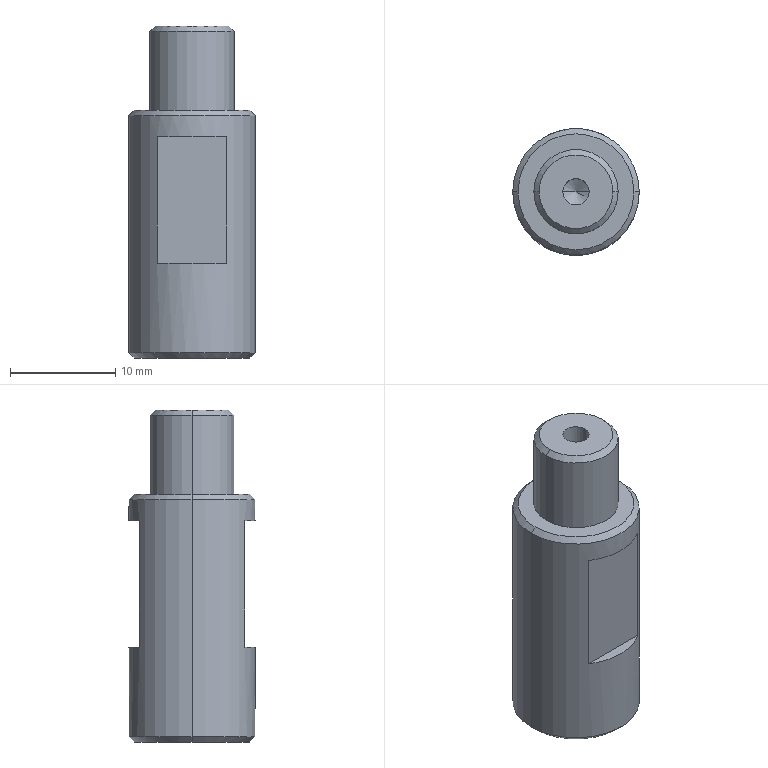Part | STEP file | 10000020542swp000-1 | 1 solid | 27 faces | box 12 x 12 x 31.5 mm | volume 2667 mm3 | cone 10 | plane 9 | cylinder 8 | commonest cylinder face diameters 2.5 x2 4.2 x2 8 x2 12 x2
STEP:
#1=CARTESIAN_POINT('',(3.5,0.,31.5));
#2=VERTEX_POINT('',#1);
#3=CARTESIAN_POINT('',(-3.5,0.,31.5));
#4=VERTEX_POINT('',#3);
#5=CARTESIAN_POINT('',(0.,0.,31.5));
#6=DIRECTION('',(0.,0.,1.));
#7=DIRECTION('',(1.,0.,0.));
#8=AXIS2_PLACEMENT_3D('',#5,#6,#7);
#9=CIRCLE('',#8,3.5);
#10=EDGE_CURVE('',#2,#4,#9,.T.);
#11=ORIENTED_EDGE('',*,*,#10,.F.);
#12=CARTESIAN_POINT('',(4.,0.,31.));
#13=VERTEX_POINT('',#12);
#14=CARTESIAN_POINT('',(3.5,0.,31.5));
#15=DIRECTION('',(0.7071,0.,-0.7071));
#16=VECTOR('',#15,1000.);
#17=LINE('',#14,#16);
#18=EDGE_CURVE('',#2,#13,#17,.T.);
#19=ORIENTED_EDGE('',*,*,#18,.T.);
#20=CARTESIAN_POINT('',(-4.,0.,31.));
#21=VERTEX_POINT('',#20);
#22=CARTESIAN_POINT('',(0.,0.,31.));
#23=DIRECTION('',(0.,0.,-1.));
#24=DIRECTION('',(1.,0.,0.));
#25=AXIS2_PLACEMENT_3D('',#22,#23,#24);
#26=CIRCLE('',#25,4.);
#27=EDGE_CURVE('',#21,#13,#26,.T.);
#28=ORIENTED_EDGE('',*,*,#27,.F.);
#29=CARTESIAN_POINT('',(-3.5,0.,31.5));
#30=DIRECTION('',(-0.7071,0.,-0.7071));
#31=VECTOR('',#30,1000.);
#32=LINE('',#29,#31);
#33=EDGE_CURVE('',#4,#21,#32,.T.);
#34=ORIENTED_EDGE('',*,*,#33,.F.);
#35=EDGE_LOOP('',(#11,#19,#28,#34));
#36=FACE_OUTER_BOUND('',#35,.T.);
#37=CARTESIAN_POINT('',(0.,0.,31.5));
#38=DIRECTION('',(0.,0.,-1.));
#39=DIRECTION('',(-1.,0.,0.));
#40=AXIS2_PLACEMENT_3D('',#37,#38,#39);
#41=CONICAL_SURFACE('',#40,3.5,0.7854);
#42=ADVANCED_FACE('',(#36),#41,.T.);
#43=CARTESIAN_POINT('',(5.5,0.,23.5));
#44=VERTEX_POINT('',#43);
#45=CARTESIAN_POINT('',(-5.5,0.,23.5));
#46=VERTEX_POINT('',#45);
#47=CARTESIAN_POINT('',(0.,0.,23.5));
#48=DIRECTION('',(0.,0.,1.));
#49=DIRECTION('',(1.,0.,0.));
#50=AXIS2_PLACEMENT_3D('',#47,#48,#49);
#51=CIRCLE('',#50,5.5);
#52=EDGE_CURVE('',#44,#46,#51,.T.);
#53=ORIENTED_EDGE('',*,*,#52,.F.);
#54=CARTESIAN_POINT('',(6.,0.,23.));
#55=VERTEX_POINT('',#54);
#56=CARTESIAN_POINT('',(5.5,0.,23.5));
#57=DIRECTION('',(0.7071,0.,-0.7071));
#58=VECTOR('',#57,1000.);
#59=LINE('',#56,#58);
#60=EDGE_CURVE('',#44,#55,#59,.T.);
#61=ORIENTED_EDGE('',*,*,#60,.T.);
#62=CARTESIAN_POINT('',(-6.,0.,23.));
#63=VERTEX_POINT('',#62);
#64=CARTESIAN_POINT('',(0.,0.,23.));
#65=DIRECTION('',(0.,0.,-1.));
#66=DIRECTION('',(1.,0.,0.));
#67=AXIS2_PLACEMENT_3D('',#64,#65,#66);
#68=CIRCLE('',#67,6.);
#69=EDGE_CURVE('',#63,#55,#68,.T.);
#70=ORIENTED_EDGE('',*,*,#69,.F.);
#71=CARTESIAN_POINT('',(-5.5,0.,23.5));
#72=DIRECTION('',(-0.7071,0.,-0.7071));
#73=VECTOR('',#72,1000.);
#74=LINE('',#71,#73);
#75=EDGE_CURVE('',#46,#63,#74,.T.);
#76=ORIENTED_EDGE('',*,*,#75,.F.);
#77=EDGE_LOOP('',(#53,#61,#70,#76));
#78=FACE_OUTER_BOUND('',#77,.T.);
#79=CARTESIAN_POINT('',(0.,0.,23.5));
#80=DIRECTION('',(0.,0.,-1.));
#81=DIRECTION('',(-1.,0.,0.));
#82=AXIS2_PLACEMENT_3D('',#79,#80,#81);
#83=CONICAL_SURFACE('',#82,5.5,0.7854);
#84=ADVANCED_FACE('',(#78),#83,.T.);
#85=CARTESIAN_POINT('',(-5.5,0.,0.));
#86=VERTEX_POINT('',#85);
#87=CARTESIAN_POINT('',(5.5,0.,0.));
#88=VERTEX_POINT('',#87);
#89=CARTESIAN_POINT('',(0.,0.,0.));
#90=DIRECTION('',(0.,0.,-1.));
#91=DIRECTION('',(1.,0.,0.));
#92=AXIS2_PLACEMENT_3D('',#89,#90,#91);
#93=CIRCLE('',#92,5.5);
#94=EDGE_CURVE('',#86,#88,#93,.T.);
#95=ORIENTED_EDGE('',*,*,#94,.F.);
#96=CARTESIAN_POINT('',(-6.,0.,0.5));
#97=VERTEX_POINT('',#96);
#98=CARTESIAN_POINT('',(-6.,0.,0.5));
#99=DIRECTION('',(-0.7071,0.,0.7071));
#100=VECTOR('',#99,1000.);
#101=LINE('',#98,#100);
#102=EDGE_CURVE('',#86,#97,#101,.T.);
#103=ORIENTED_EDGE('',*,*,#102,.T.);
#104=CARTESIAN_POINT('',(6.,0.,0.5));
#105=VERTEX_POINT('',#104);
#106=CARTESIAN_POINT('',(0.,0.,0.5));
#107=DIRECTION('',(0.,0.,1.));
#108=DIRECTION('',(1.,0.,0.));
#109=AXIS2_PLACEMENT_3D('',#106,#107,#108);
#110=CIRCLE('',#109,6.);
#111=EDGE_CURVE('',#105,#97,#110,.T.);
#112=ORIENTED_EDGE('',*,*,#111,.F.);
#113=CARTESIAN_POINT('',(6.,0.,0.5));
#114=DIRECTION('',(0.7071,0.,0.7071));
#115=VECTOR('',#114,1000.);
#116=LINE('',#113,#115);
#117=EDGE_CURVE('',#88,#105,#116,.T.);
#118=ORIENTED_EDGE('',*,*,#117,.F.);
#119=EDGE_LOOP('',(#95,#103,#112,#118));
#120=FACE_OUTER_BOUND('',#119,.T.);
#121=CARTESIAN_POINT('',(0.,0.,0.5));
#122=DIRECTION('',(0.,0.,1.));
#123=DIRECTION('',(1.,0.,0.));
#124=AXIS2_PLACEMENT_3D('',#121,#122,#123);
#125=CONICAL_SURFACE('',#124,6.,0.7854);
#126=ADVANCED_FACE('',(#120),#125,.T.);
#127=CARTESIAN_POINT('',(2.1,0.,14.4));
#128=VERTEX_POINT('',#127);
#129=CARTESIAN_POINT('',(-2.1,0.,14.4));
#130=VERTEX_POINT('',#129);
#131=CARTESIAN_POINT('',(0.,0.,14.4));
#132=DIRECTION('',(0.,0.,-1.));
#133=DIRECTION('',(-1.,0.,0.));
#134=AXIS2_PLACEMENT_3D('',#131,#132,#133);
#135=CIRCLE('',#134,2.1);
#136=EDGE_CURVE('',#128,#130,#135,.T.);
#137=ORIENTED_EDGE('',*,*,#136,.F.);
#138=CARTESIAN_POINT('',(2.1,0.,0.));
#139=VERTEX_POINT('',#138);
#140=CARTESIAN_POINT('',(2.1,0.,0.));
#141=DIRECTION('',(0.,0.,-1.));
#142=VECTOR('',#141,1000.);
#143=LINE('',#140,#142);
#144=EDGE_CURVE('',#128,#139,#143,.T.);
#145=ORIENTED_EDGE('',*,*,#144,.T.);
#146=CARTESIAN_POINT('',(-2.1,0.,0.));
#147=VERTEX_POINT('',#146);
#148=CARTESIAN_POINT('',(0.,0.,0.));
#149=DIRECTION('',(0.,0.,-1.));
#150=DIRECTION('',(-1.,0.,0.));
#151=AXIS2_PLACEMENT_3D('',#148,#149,#150);
#152=CIRCLE('',#151,2.1);
#153=EDGE_CURVE('',#139,#147,#152,.T.);
#154=ORIENTED_EDGE('',*,*,#153,.T.);
#155=CARTESIAN_POINT('',(-2.1,0.,0.));
#156=DIRECTION('',(0.,0.,-1.));
#157=VECTOR('',#156,1000.);
#158=LINE('',#155,#157);
#159=EDGE_CURVE('',#130,#147,#158,.T.);
#160=ORIENTED_EDGE('',*,*,#159,.F.);
#161=EDGE_LOOP('',(#137,#145,#154,#160));
#162=FACE_OUTER_BOUND('',#161,.T.);
#163=CARTESIAN_POINT('',(0.,0.,0.));
#164=DIRECTION('',(0.,0.,-1.));
#165=DIRECTION('',(-1.,0.,0.));
#166=AXIS2_PLACEMENT_3D('',#163,#164,#165);
#167=CYLINDRICAL_SURFACE('',#166,2.1);
#168=ADVANCED_FACE('',(#162),#167,.F.);
#169=CARTESIAN_POINT('',(0.,0.,15.662));
#170=VERTEX_POINT('',#169);
#171=CARTESIAN_POINT('',(-2.1,0.,14.4));
#172=DIRECTION('',(-0.8572,0.,-0.515));
#173=VECTOR('',#172,1000.);
#174=LINE('',#171,#173);
#175=EDGE_CURVE('',#170,#130,#174,.T.);
#176=ORIENTED_EDGE('',*,*,#175,.F.);
#177=CARTESIAN_POINT('',(2.1,0.,14.4));
#178=DIRECTION('',(0.8572,0.,-0.515));
#179=VECTOR('',#178,1000.);
#180=LINE('',#177,#179);
#181=EDGE_CURVE('',#170,#128,#180,.T.);
#182=ORIENTED_EDGE('',*,*,#181,.T.);
#183=ORIENTED_EDGE('',*,*,#136,.T.);
#184=EDGE_LOOP('',(#176,#182,#183));
#185=FACE_OUTER_BOUND('',#184,.T.);
#186=CARTESIAN_POINT('',(0.,0.,14.4));
#187=DIRECTION('',(0.,0.,-1.));
#188=DIRECTION('',(-1.,0.,0.));
#189=AXIS2_PLACEMENT_3D('',#186,#187,#188);
#190=CONICAL_SURFACE('',#189,2.1,1.03);
#191=ADVANCED_FACE('',(#185),#190,.F.);
#192=CARTESIAN_POINT('',(-1.25,0.,18.));
#193=VERTEX_POINT('',#192);
#194=CARTESIAN_POINT('',(1.25,0.,18.));
#195=VERTEX_POINT('',#194);
#196=CARTESIAN_POINT('',(0.,0.,18.));
#197=DIRECTION('',(0.,0.,1.));
#198=DIRECTION('',(1.,0.,0.));
#199=AXIS2_PLACEMENT_3D('',#196,#197,#198);
#200=CIRCLE('',#199,1.25);
#201=EDGE_CURVE('',#193,#195,#200,.T.);
#202=ORIENTED_EDGE('',*,*,#201,.F.);
#203=CARTESIAN_POINT('',(-1.25,0.,31.5));
#204=VERTEX_POINT('',#203);
#205=CARTESIAN_POINT('',(-1.25,0.,31.5));
#206=DIRECTION('',(0.,0.,1.));
#207=VECTOR('',#206,1000.);
#208=LINE('',#205,#207);
#209=EDGE_CURVE('',#193,#204,#208,.T.);
#210=ORIENTED_EDGE('',*,*,#209,.T.);
#211=CARTESIAN_POINT('',(1.25,0.,31.5));
#212=VERTEX_POINT('',#211);
#213=CARTESIAN_POINT('',(0.,0.,31.5));
#214=DIRECTION('',(0.,0.,1.));
#215=DIRECTION('',(1.,0.,0.));
#216=AXIS2_PLACEMENT_3D('',#213,#214,#215);
#217=CIRCLE('',#216,1.25);
#218=EDGE_CURVE('',#204,#212,#217,.T.);
#219=ORIENTED_EDGE('',*,*,#218,.T.);
#220=CARTESIAN_POINT('',(1.25,0.,31.5));
#221=DIRECTION('',(0.,0.,1.));
#222=VECTOR('',#221,1000.);
#223=LINE('',#220,#222);
#224=EDGE_CURVE('',#195,#212,#223,.T.);
#225=ORIENTED_EDGE('',*,*,#224,.F.);
#226=EDGE_LOOP('',(#202,#210,#219,#225));
#227=FACE_OUTER_BOUND('',#226,.T.);
#228=CARTESIAN_POINT('',(0.,0.,31.5));
#229=DIRECTION('',(0.,0.,1.));
#230=DIRECTION('',(1.,0.,0.));
#231=AXIS2_PLACEMENT_3D('',#228,#229,#230);
#232=CYLINDRICAL_SURFACE('',#231,1.25);
#233=ADVANCED_FACE('',(#227),#232,.F.);
#234=CARTESIAN_POINT('',(0.,0.,17.249));
#235=VERTEX_POINT('',#234);
#236=CARTESIAN_POINT('',(1.25,0.,18.));
#237=DIRECTION('',(0.8572,0.,0.515));
#238=VECTOR('',#237,1000.);
#239=LINE('',#236,#238);
#240=EDGE_CURVE('',#235,#195,#239,.T.);
#241=ORIENTED_EDGE('',*,*,#240,.F.);
#242=CARTESIAN_POINT('',(-1.25,0.,18.));
#243=DIRECTION('',(-0.8572,0.,0.515));
#244=VECTOR('',#243,1000.);
#245=LINE('',#242,#244);
#246=EDGE_CURVE('',#235,#193,#245,.T.);
#247=ORIENTED_EDGE('',*,*,#246,.T.);
#248=ORIENTED_EDGE('',*,*,#201,.T.);
#249=EDGE_LOOP('',(#241,#247,#248));
#250=FACE_OUTER_BOUND('',#249,.T.);
#251=CARTESIAN_POINT('',(0.,0.,18.));
#252=DIRECTION('',(0.,0.,1.));
#253=DIRECTION('',(1.,0.,0.));
#254=AXIS2_PLACEMENT_3D('',#251,#252,#253);
#255=CONICAL_SURFACE('',#254,1.25,1.03);
#256=ADVANCED_FACE('',(#250),#255,.F.);
#257=ORIENTED_EDGE('',*,*,#27,.T.);
#258=CARTESIAN_POINT('',(4.,0.,23.5));
#259=VERTEX_POINT('',#258);
#260=CARTESIAN_POINT('',(4.,0.,31.5));
#261=DIRECTION('',(0.,0.,-1.));
#262=VECTOR('',#261,1000.);
#263=LINE('',#260,#262);
#264=EDGE_CURVE('',#13,#259,#263,.T.);
#265=ORIENTED_EDGE('',*,*,#264,.T.);
#266=CARTESIAN_POINT('',(-4.,0.,23.5));
#267=VERTEX_POINT('',#266);
#268=CARTESIAN_POINT('',(0.,0.,23.5));
#269=DIRECTION('',(0.,0.,1.));
#270=DIRECTION('',(1.,0.,0.));
#271=AXIS2_PLACEMENT_3D('',#268,#269,#270);
#272=CIRCLE('',#271,4.);
#273=EDGE_CURVE('',#259,#267,#272,.T.);
#274=ORIENTED_EDGE('',*,*,#273,.T.);
#275=CARTESIAN_POINT('',(-4.,0.,31.5));
#276=DIRECTION('',(0.,0.,-1.));
#277=VECTOR('',#276,1000.);
#278=LINE('',#275,#277);
#279=EDGE_CURVE('',#21,#267,#278,.T.);
#280=ORIENTED_EDGE('',*,*,#279,.F.);
#281=EDGE_LOOP('',(#257,#265,#274,#280));
#282=FACE_OUTER_BOUND('',#281,.T.);
#283=CARTESIAN_POINT('',(0.,0.,31.5));
#284=DIRECTION('',(0.,0.,-1.));
#285=DIRECTION('',(-1.,0.,0.));
#286=AXIS2_PLACEMENT_3D('',#283,#284,#285);
#287=CYLINDRICAL_SURFACE('',#286,4.);
#288=ADVANCED_FACE('',(#282),#287,.T.);
#289=CARTESIAN_POINT('',(3.317,5.,21.));
#290=VERTEX_POINT('',#289);
#291=CARTESIAN_POINT('',(3.317,5.,9.));
#292=VERTEX_POINT('',#291);
#293=CARTESIAN_POINT('',(3.317,5.,23.5));
#294=DIRECTION('',(0.,0.,-1.));
#295=VECTOR('',#294,1000.);
#296=LINE('',#293,#295);
#297=EDGE_CURVE('',#290,#292,#296,.T.);
#298=ORIENTED_EDGE('',*,*,#297,.F.);
#299=CARTESIAN_POINT('',(-3.317,5.,21.));
#300=VERTEX_POINT('',#299);
#301=CARTESIAN_POINT('',(0.,0.,21.));
#302=DIRECTION('',(0.,0.,-1.));
#303=DIRECTION('',(-1.,0.,0.));
#304=AXIS2_PLACEMENT_3D('',#301,#302,#303);
#305=CIRCLE('',#304,6.);
#306=EDGE_CURVE('',#300,#290,#305,.T.);
#307=ORIENTED_EDGE('',*,*,#306,.F.);
#308=CARTESIAN_POINT('',(-3.317,5.,9.));
#309=VERTEX_POINT('',#308);
#310=CARTESIAN_POINT('',(-3.317,5.,23.5));
#311=DIRECTION('',(0.,0.,1.));
#312=VECTOR('',#311,1000.);
#313=LINE('',#310,#312);
#314=EDGE_CURVE('',#309,#300,#313,.T.);
#315=ORIENTED_EDGE('',*,*,#314,.F.);
#316=CARTESIAN_POINT('',(0.,0.,9.));
#317=DIRECTION('',(0.,0.,1.));
#318=DIRECTION('',(1.,0.,0.));
#319=AXIS2_PLACEMENT_3D('',#316,#317,#318);
#320=CIRCLE('',#319,6.);
#321=EDGE_CURVE('',#292,#309,#320,.T.);
#322=ORIENTED_EDGE('',*,*,#321,.F.);
#323=EDGE_LOOP('',(#298,#307,#315,#322));
#324=FACE_BOUND('',#323,.T.);
#325=ORIENTED_EDGE('',*,*,#69,.T.);
#326=CARTESIAN_POINT('',(6.,0.,23.5));
#327=DIRECTION('',(0.,0.,-1.));
#328=VECTOR('',#327,1000.);
#329=LINE('',#326,#328);
#330=EDGE_CURVE('',#55,#105,#329,.T.);
#331=ORIENTED_EDGE('',*,*,#330,.T.);
#332=ORIENTED_EDGE('',*,*,#111,.T.);
#333=CARTESIAN_POINT('',(-6.,0.,23.5));
#334=DIRECTION('',(0.,0.,-1.));
#335=VECTOR('',#334,1000.);
#336=LINE('',#333,#335);
#337=EDGE_CURVE('',#63,#97,#336,.T.);
#338=ORIENTED_EDGE('',*,*,#337,.F.);
#339=EDGE_LOOP('',(#325,#331,#332,#338));
#340=FACE_OUTER_BOUND('',#339,.T.);
#341=CARTESIAN_POINT('',(0.,0.,23.5));
#342=DIRECTION('',(0.,0.,-1.));
#343=DIRECTION('',(-1.,0.,0.));
#344=AXIS2_PLACEMENT_3D('',#341,#342,#343);
#345=CYLINDRICAL_SURFACE('',#344,6.);
#346=ADVANCED_FACE('',(#324,#340),#345,.T.);
#347=ORIENTED_EDGE('',*,*,#330,.F.);
#348=CARTESIAN_POINT('',(0.,0.,23.));
#349=DIRECTION('',(0.,0.,-1.));
#350=DIRECTION('',(1.,0.,0.));
#351=AXIS2_PLACEMENT_3D('',#348,#349,#350);
#352=CIRCLE('',#351,6.);
#353=EDGE_CURVE('',#55,#63,#352,.T.);
#354=ORIENTED_EDGE('',*,*,#353,.T.);
#355=ORIENTED_EDGE('',*,*,#337,.T.);
#356=CARTESIAN_POINT('',(0.,0.,0.5));
#357=DIRECTION('',(0.,0.,1.));
#358=DIRECTION('',(1.,0.,0.));
#359=AXIS2_PLACEMENT_3D('',#356,#357,#358);
#360=CIRCLE('',#359,6.);
#361=EDGE_CURVE('',#97,#105,#360,.T.);
#362=ORIENTED_EDGE('',*,*,#361,.T.);
#363=EDGE_LOOP('',(#347,#354,#355,#362));
#364=FACE_OUTER_BOUND('',#363,.T.);
#365=CARTESIAN_POINT('',(-3.317,-5.,21.));
#366=VERTEX_POINT('',#365);
#367=CARTESIAN_POINT('',(-3.317,-5.,9.));
#368=VERTEX_POINT('',#367);
#369=CARTESIAN_POINT('',(-3.317,-5.,23.5));
#370=DIRECTION('',(0.,0.,-1.));
#371=VECTOR('',#370,1000.);
#372=LINE('',#369,#371);
#373=EDGE_CURVE('',#366,#368,#372,.T.);
#374=ORIENTED_EDGE('',*,*,#373,.F.);
#375=CARTESIAN_POINT('',(3.317,-5.,21.));
#376=VERTEX_POINT('',#375);
#377=CARTESIAN_POINT('',(0.,0.,21.));
#378=DIRECTION('',(0.,0.,1.));
#379=DIRECTION('',(1.,0.,0.));
#380=AXIS2_PLACEMENT_3D('',#377,#378,#379);
#381=CIRCLE('',#380,6.);
#382=EDGE_CURVE('',#366,#376,#381,.T.);
#383=ORIENTED_EDGE('',*,*,#382,.T.);
#384=CARTESIAN_POINT('',(3.317,-5.,9.));
#385=VERTEX_POINT('',#384);
#386=CARTESIAN_POINT('',(3.317,-5.,23.5));
#387=DIRECTION('',(0.,0.,1.));
#388=VECTOR('',#387,1000.);
#389=LINE('',#386,#388);
#390=EDGE_CURVE('',#385,#376,#389,.T.);
#391=ORIENTED_EDGE('',*,*,#390,.F.);
#392=CARTESIAN_POINT('',(0.,0.,9.));
#393=DIRECTION('',(0.,0.,-1.));
#394=DIRECTION('',(-1.,0.,0.));
#395=AXIS2_PLACEMENT_3D('',#392,#393,#394);
#396=CIRCLE('',#395,6.);
#397=EDGE_CURVE('',#385,#368,#396,.T.);
#398=ORIENTED_EDGE('',*,*,#397,.T.);
#399=EDGE_LOOP('',(#374,#383,#391,#398));
#400=FACE_BOUND('',#399,.T.);
#401=CARTESIAN_POINT('',(0.,0.,23.5));
#402=DIRECTION('',(0.,0.,-1.));
#403=DIRECTION('',(-1.,0.,0.));
#404=AXIS2_PLACEMENT_3D('',#401,#402,#403);
#405=CYLINDRICAL_SURFACE('',#404,6.);
#406=ADVANCED_FACE('',(#364,#400),#405,.T.);
#407=CARTESIAN_POINT('',(0.,0.,23.5));
#408=DIRECTION('',(0.,0.,1.));
#409=DIRECTION('',(1.,0.,0.));
#410=AXIS2_PLACEMENT_3D('',#407,#408,#409);
#411=CIRCLE('',#410,5.5);
#412=EDGE_CURVE('',#46,#44,#411,.T.);
#413=ORIENTED_EDGE('',*,*,#412,.T.);
#414=ORIENTED_EDGE('',*,*,#52,.T.);
#415=EDGE_LOOP('',(#413,#414));
#416=FACE_OUTER_BOUND('',#415,.T.);
#417=CARTESIAN_POINT('',(0.,0.,23.5));
#418=DIRECTION('',(0.,0.,1.));
#419=DIRECTION('',(1.,0.,0.));
#420=AXIS2_PLACEMENT_3D('',#417,#418,#419);
#421=CIRCLE('',#420,4.);
#422=EDGE_CURVE('',#267,#259,#421,.T.);
#423=ORIENTED_EDGE('',*,*,#422,.F.);
#424=ORIENTED_EDGE('',*,*,#273,.F.);
#425=EDGE_LOOP('',(#423,#424));
#426=FACE_BOUND('',#425,.T.);
#427=CARTESIAN_POINT('',(0.,0.,23.5));
#428=DIRECTION('',(0.,0.,1.));
#429=DIRECTION('',(1.,0.,0.));
#430=AXIS2_PLACEMENT_3D('',#427,#428,#429);
#431=PLANE('',#430);
#432=ADVANCED_FACE('',(#416,#426),#431,.T.);
#433=CARTESIAN_POINT('',(0.,0.,0.));
#434=DIRECTION('',(0.,0.,-1.));
#435=DIRECTION('',(1.,0.,0.));
#436=AXIS2_PLACEMENT_3D('',#433,#434,#435);
#437=CIRCLE('',#436,5.5);
#438=EDGE_CURVE('',#88,#86,#437,.T.);
#439=ORIENTED_EDGE('',*,*,#438,.T.);
#440=ORIENTED_EDGE('',*,*,#94,.T.);
#441=EDGE_LOOP('',(#439,#440));
#442=FACE_OUTER_BOUND('',#441,.T.);
#443=CARTESIAN_POINT('',(0.,0.,0.));
#444=DIRECTION('',(0.,0.,-1.));
#445=DIRECTION('',(-1.,0.,0.));
#446=AXIS2_PLACEMENT_3D('',#443,#444,#445);
#447=CIRCLE('',#446,2.1);
#448=EDGE_CURVE('',#147,#139,#447,.T.);
#449=ORIENTED_EDGE('',*,*,#448,.F.);
#450=ORIENTED_EDGE('',*,*,#153,.F.);
#451=EDGE_LOOP('',(#449,#450));
#452=FACE_BOUND('',#451,.T.);
#453=CARTESIAN_POINT('',(0.,0.,0.));
#454=DIRECTION('',(0.,0.,1.));
#455=DIRECTION('',(1.,0.,0.));
#456=AXIS2_PLACEMENT_3D('',#453,#454,#455);
#457=PLANE('',#456);
#458=ADVANCED_FACE('',(#442,#452),#457,.F.);
#459=ORIENTED_EDGE('',*,*,#264,.F.);
#460=CARTESIAN_POINT('',(0.,0.,31.));
#461=DIRECTION('',(0.,0.,-1.));
#462=DIRECTION('',(1.,0.,0.));
#463=AXIS2_PLACEMENT_3D('',#460,#461,#462);
#464=CIRCLE('',#463,4.);
#465=EDGE_CURVE('',#13,#21,#464,.T.);
#466=ORIENTED_EDGE('',*,*,#465,.T.);
#467=ORIENTED_EDGE('',*,*,#279,.T.);
#468=ORIENTED_EDGE('',*,*,#422,.T.);
#469=EDGE_LOOP('',(#459,#466,#467,#468));
#470=FACE_OUTER_BOUND('',#469,.T.);
#471=CARTESIAN_POINT('',(0.,0.,31.5));
#472=DIRECTION('',(0.,0.,-1.));
#473=DIRECTION('',(-1.,0.,0.));
#474=AXIS2_PLACEMENT_3D('',#471,#472,#473);
#475=CYLINDRICAL_SURFACE('',#474,4.);
#476=ADVANCED_FACE('',(#470),#475,.T.);
#477=CARTESIAN_POINT('',(0.,0.,31.5));
#478=DIRECTION('',(0.,0.,1.));
#479=DIRECTION('',(1.,0.,0.));
#480=AXIS2_PLACEMENT_3D('',#477,#478,#479);
#481=CIRCLE('',#480,3.5);
#482=EDGE_CURVE('',#4,#2,#481,.T.);
#483=ORIENTED_EDGE('',*,*,#482,.T.);
#484=ORIENTED_EDGE('',*,*,#10,.T.);
#485=EDGE_LOOP('',(#483,#484));
#486=FACE_OUTER_BOUND('',#485,.T.);
#487=CARTESIAN_POINT('',(0.,0.,31.5));
#488=DIRECTION('',(0.,0.,1.));
#489=DIRECTION('',(1.,0.,0.));
#490=AXIS2_PLACEMENT_3D('',#487,#488,#489);
#491=CIRCLE('',#490,1.25);
#492=EDGE_CURVE('',#212,#204,#491,.T.);
#493=ORIENTED_EDGE('',*,*,#492,.F.);
#494=ORIENTED_EDGE('',*,*,#218,.F.);
#495=EDGE_LOOP('',(#493,#494));
#496=FACE_BOUND('',#495,.T.);
#497=CARTESIAN_POINT('',(0.,0.,31.5));
#498=DIRECTION('',(0.,0.,1.));
#499=DIRECTION('',(1.,0.,0.));
#500=AXIS2_PLACEMENT_3D('',#497,#498,#499);
#501=PLANE('',#500);
#502=ADVANCED_FACE('',(#486,#496),#501,.T.);
#503=ORIENTED_EDGE('',*,*,#306,.T.);
#504=CARTESIAN_POINT('',(-7.036,5.,21.));
#505=DIRECTION('',(1.,0.,0.));
#506=VECTOR('',#505,1000.);
#507=LINE('',#504,#506);
#508=EDGE_CURVE('',#300,#290,#507,.T.);
#509=ORIENTED_EDGE('',*,*,#508,.F.);
#510=EDGE_LOOP('',(#503,#509));
#511=FACE_OUTER_BOUND('',#510,.T.);
#512=CARTESIAN_POINT('',(-7.036,13.,21.));
#513=DIRECTION('',(0.,0.,-1.));
#514=DIRECTION('',(-1.,0.,0.));
#515=AXIS2_PLACEMENT_3D('',#512,#513,#514);
#516=PLANE('',#515);
#517=ADVANCED_FACE('',(#511),#516,.T.);
#518=ORIENTED_EDGE('',*,*,#321,.T.);
#519=CARTESIAN_POINT('',(-7.036,5.,9.));
#520=DIRECTION('',(-1.,0.,0.));
#521=VECTOR('',#520,1000.);
#522=LINE('',#519,#521);
#523=EDGE_CURVE('',#292,#309,#522,.T.);
#524=ORIENTED_EDGE('',*,*,#523,.F.);
#525=EDGE_LOOP('',(#518,#524));
#526=FACE_OUTER_BOUND('',#525,.T.);
#527=CARTESIAN_POINT('',(-7.036,13.,9.));
#528=DIRECTION('',(0.,0.,1.));
#529=DIRECTION('',(1.,0.,0.));
#530=AXIS2_PLACEMENT_3D('',#527,#528,#529);
#531=PLANE('',#530);
#532=ADVANCED_FACE('',(#526),#531,.T.);
#533=ORIENTED_EDGE('',*,*,#297,.T.);
#534=ORIENTED_EDGE('',*,*,#523,.T.);
#535=ORIENTED_EDGE('',*,*,#314,.T.);
#536=ORIENTED_EDGE('',*,*,#508,.T.);
#537=EDGE_LOOP('',(#533,#534,#535,#536));
#538=FACE_OUTER_BOUND('',#537,.T.);
#539=CARTESIAN_POINT('',(0.,5.,0.));
#540=DIRECTION('',(0.,1.,0.));
#541=DIRECTION('',(0.,0.,1.));
#542=AXIS2_PLACEMENT_3D('',#539,#540,#541);
#543=PLANE('',#542);
#544=ADVANCED_FACE('',(#538),#543,.T.);
#545=CARTESIAN_POINT('',(-7.036,-5.,9.));
#546=DIRECTION('',(-1.,0.,0.));
#547=VECTOR('',#546,1000.);
#548=LINE('',#545,#547);
#549=EDGE_CURVE('',#385,#368,#548,.T.);
#550=ORIENTED_EDGE('',*,*,#549,.T.);
#551=ORIENTED_EDGE('',*,*,#397,.F.);
#552=EDGE_LOOP('',(#550,#551));
#553=FACE_OUTER_BOUND('',#552,.T.);
#554=CARTESIAN_POINT('',(-7.036,-13.,9.));
#555=DIRECTION('',(0.,0.,-1.));
#556=DIRECTION('',(-1.,0.,0.));
#557=AXIS2_PLACEMENT_3D('',#554,#555,#556);
#558=PLANE('',#557);
#559=ADVANCED_FACE('',(#553),#558,.F.);
#560=CARTESIAN_POINT('',(-7.036,-5.,21.));
#561=DIRECTION('',(1.,0.,0.));
#562=VECTOR('',#561,1000.);
#563=LINE('',#560,#562);
#564=EDGE_CURVE('',#366,#376,#563,.T.);
#565=ORIENTED_EDGE('',*,*,#564,.T.);
#566=ORIENTED_EDGE('',*,*,#382,.F.);
#567=EDGE_LOOP('',(#565,#566));
#568=FACE_OUTER_BOUND('',#567,.T.);
#569=CARTESIAN_POINT('',(-7.036,-13.,21.));
#570=DIRECTION('',(0.,0.,1.));
#571=DIRECTION('',(1.,0.,0.));
#572=AXIS2_PLACEMENT_3D('',#569,#570,#571);
#573=PLANE('',#572);
#574=ADVANCED_FACE('',(#568),#573,.F.);
#575=ORIENTED_EDGE('',*,*,#373,.T.);
#576=ORIENTED_EDGE('',*,*,#549,.F.);
#577=ORIENTED_EDGE('',*,*,#390,.T.);
#578=ORIENTED_EDGE('',*,*,#564,.F.);
#579=EDGE_LOOP('',(#575,#576,#577,#578));
#580=FACE_OUTER_BOUND('',#579,.T.);
#581=CARTESIAN_POINT('',(0.,-5.,0.));
#582=DIRECTION('',(0.,-1.,0.));
#583=DIRECTION('',(0.,0.,1.));
#584=AXIS2_PLACEMENT_3D('',#581,#582,#583);
#585=PLANE('',#584);
#586=ADVANCED_FACE('',(#580),#585,.T.);
#587=ORIENTED_EDGE('',*,*,#246,.F.);
#588=ORIENTED_EDGE('',*,*,#240,.T.);
#589=CARTESIAN_POINT('',(0.,0.,18.));
#590=DIRECTION('',(0.,0.,1.));
#591=DIRECTION('',(1.,0.,0.));
#592=AXIS2_PLACEMENT_3D('',#589,#590,#591);
#593=CIRCLE('',#592,1.25);
#594=EDGE_CURVE('',#195,#193,#593,.T.);
#595=ORIENTED_EDGE('',*,*,#594,.T.);
#596=EDGE_LOOP('',(#587,#588,#595));
#597=FACE_OUTER_BOUND('',#596,.T.);
#598=CARTESIAN_POINT('',(0.,0.,18.));
#599=DIRECTION('',(0.,0.,1.));
#600=DIRECTION('',(1.,0.,0.));
#601=AXIS2_PLACEMENT_3D('',#598,#599,#600);
#602=CONICAL_SURFACE('',#601,1.25,1.03);
#603=ADVANCED_FACE('',(#597),#602,.F.);
#604=ORIENTED_EDGE('',*,*,#209,.F.);
#605=ORIENTED_EDGE('',*,*,#594,.F.);
#606=ORIENTED_EDGE('',*,*,#224,.T.);
#607=ORIENTED_EDGE('',*,*,#492,.T.);
#608=EDGE_LOOP('',(#604,#605,#606,#607));
#609=FACE_OUTER_BOUND('',#608,.T.);
#610=CARTESIAN_POINT('',(0.,0.,31.5));
#611=DIRECTION('',(0.,0.,1.));
#612=DIRECTION('',(1.,0.,0.));
#613=AXIS2_PLACEMENT_3D('',#610,#611,#612);
#614=CYLINDRICAL_SURFACE('',#613,1.25);
#615=ADVANCED_FACE('',(#609),#614,.F.);
#616=ORIENTED_EDGE('',*,*,#181,.F.);
#617=ORIENTED_EDGE('',*,*,#175,.T.);
#618=CARTESIAN_POINT('',(0.,0.,14.4));
#619=DIRECTION('',(0.,0.,-1.));
#620=DIRECTION('',(-1.,0.,0.));
#621=AXIS2_PLACEMENT_3D('',#618,#619,#620);
#622=CIRCLE('',#621,2.1);
#623=EDGE_CURVE('',#130,#128,#622,.T.);
#624=ORIENTED_EDGE('',*,*,#623,.T.);
#625=EDGE_LOOP('',(#616,#617,#624));
#626=FACE_OUTER_BOUND('',#625,.T.);
#627=CARTESIAN_POINT('',(0.,0.,14.4));
#628=DIRECTION('',(0.,0.,-1.));
#629=DIRECTION('',(-1.,0.,0.));
#630=AXIS2_PLACEMENT_3D('',#627,#628,#629);
#631=CONICAL_SURFACE('',#630,2.1,1.03);
#632=ADVANCED_FACE('',(#626),#631,.F.);
#633=ORIENTED_EDGE('',*,*,#144,.F.);
#634=ORIENTED_EDGE('',*,*,#623,.F.);
#635=ORIENTED_EDGE('',*,*,#159,.T.);
#636=ORIENTED_EDGE('',*,*,#448,.T.);
#637=EDGE_LOOP('',(#633,#634,#635,#636));
#638=FACE_OUTER_BOUND('',#637,.T.);
#639=CARTESIAN_POINT('',(0.,0.,0.));
#640=DIRECTION('',(0.,0.,-1.));
#641=DIRECTION('',(-1.,0.,0.));
#642=AXIS2_PLACEMENT_3D('',#639,#640,#641);
#643=CYLINDRICAL_SURFACE('',#642,2.1);
#644=ADVANCED_FACE('',(#638),#643,.F.);
#645=ORIENTED_EDGE('',*,*,#102,.F.);
#646=ORIENTED_EDGE('',*,*,#438,.F.);
#647=ORIENTED_EDGE('',*,*,#117,.T.);
#648=ORIENTED_EDGE('',*,*,#361,.F.);
#649=EDGE_LOOP('',(#645,#646,#647,#648));
#650=FACE_OUTER_BOUND('',#649,.T.);
#651=CARTESIAN_POINT('',(0.,0.,0.5));
#652=DIRECTION('',(0.,0.,1.));
#653=DIRECTION('',(1.,0.,0.));
#654=AXIS2_PLACEMENT_3D('',#651,#652,#653);
#655=CONICAL_SURFACE('',#654,6.,0.7854);
#656=ADVANCED_FACE('',(#650),#655,.T.);
#657=ORIENTED_EDGE('',*,*,#60,.F.);
#658=ORIENTED_EDGE('',*,*,#412,.F.);
#659=ORIENTED_EDGE('',*,*,#75,.T.);
#660=ORIENTED_EDGE('',*,*,#353,.F.);
#661=EDGE_LOOP('',(#657,#658,#659,#660));
#662=FACE_OUTER_BOUND('',#661,.T.);
#663=CARTESIAN_POINT('',(0.,0.,23.5));
#664=DIRECTION('',(0.,0.,-1.));
#665=DIRECTION('',(-1.,0.,0.));
#666=AXIS2_PLACEMENT_3D('',#663,#664,#665);
#667=CONICAL_SURFACE('',#666,5.5,0.7854);
#668=ADVANCED_FACE('',(#662),#667,.T.);
#669=ORIENTED_EDGE('',*,*,#18,.F.);
#670=ORIENTED_EDGE('',*,*,#482,.F.);
#671=ORIENTED_EDGE('',*,*,#33,.T.);
#672=ORIENTED_EDGE('',*,*,#465,.F.);
#673=EDGE_LOOP('',(#669,#670,#671,#672));
#674=FACE_OUTER_BOUND('',#673,.T.);
#675=CARTESIAN_POINT('',(0.,0.,31.5));
#676=DIRECTION('',(0.,0.,-1.));
#677=DIRECTION('',(-1.,0.,0.));
#678=AXIS2_PLACEMENT_3D('',#675,#676,#677);
#679=CONICAL_SURFACE('',#678,3.5,0.7854);
#680=ADVANCED_FACE('',(#674),#679,.T.);
#681=CLOSED_SHELL('',(#42,#84,#126,#168,#191,#233,#256,#288,#346,#406,#432,#458,#476,#502,#517,#532,#544,#559,#574,#586,#603,#615,#632,#644,#656,#668,#680));
#682=MANIFOLD_SOLID_BREP('',#681);
#683=CARTESIAN_POINT('',(0.,0.,0.));
#684=DIRECTION('',(0.,0.,1.));
#685=DIRECTION('',(1.,0.,0.));
#686=AXIS2_PLACEMENT_3D('',#683,#684,#685);
#687=(LENGTH_UNIT()NAMED_UNIT(*)SI_UNIT(.MILLI.,.METRE.));
#688=UNCERTAINTY_MEASURE_WITH_UNIT(LENGTH_MEASURE(0.00001),#687,'','');
#689=(NAMED_UNIT(*)PLANE_ANGLE_UNIT()SI_UNIT($,.RADIAN.));
#690=(NAMED_UNIT(*)SI_UNIT($,.STERADIAN.)SOLID_ANGLE_UNIT());
#691=(GEOMETRIC_REPRESENTATION_CONTEXT(3)GLOBAL_UNCERTAINTY_ASSIGNED_CONTEXT((#688))GLOBAL_UNIT_ASSIGNED_CONTEXT((#687,#689,#690))REPRESENTATION_CONTEXT('',''));
#692=ADVANCED_BREP_SHAPE_REPRESENTATION('',(#682,#686),#691);